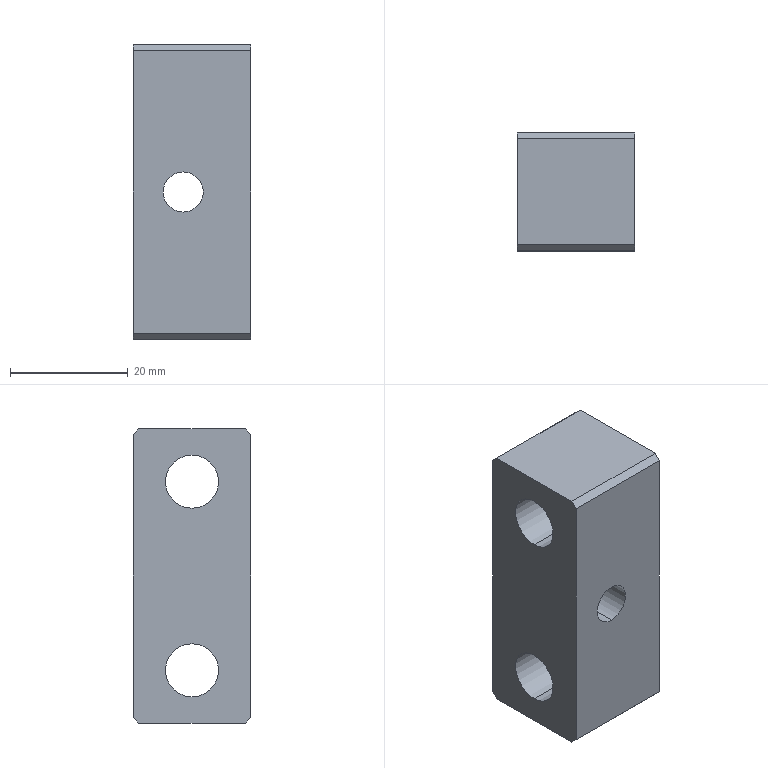Part | STEP file | PN_0010 Block_Default | 1 solid | 22 faces | box 20 x 20 x 50 mm | volume 14883 mm3 | plane 12 | cylinder 10 | commonest cylinder face diameters 9 x4 14 x4 6.8 x2